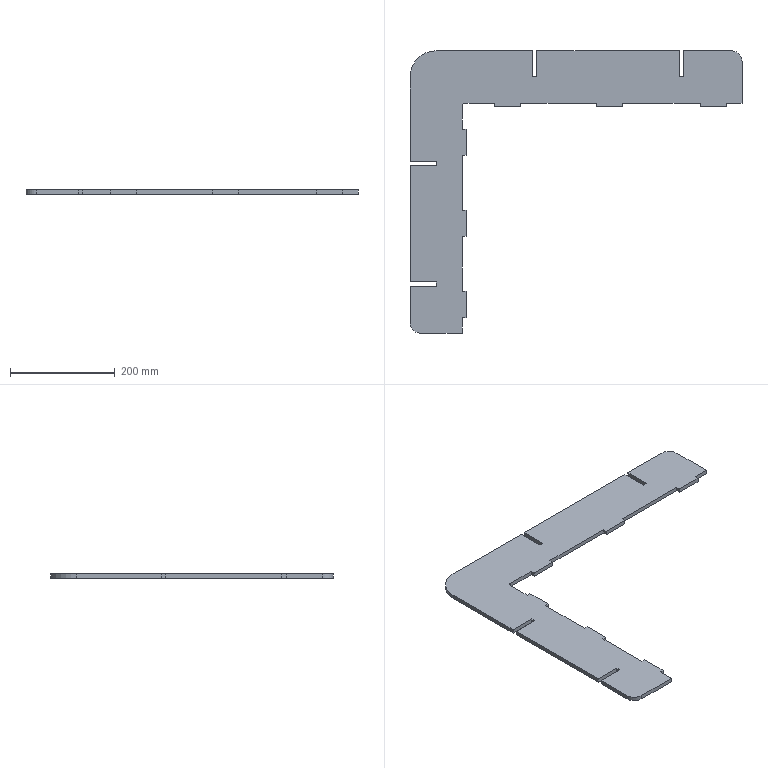Part | SolidWorks | features FlatPattern 1, SMBaseFlange 1, SheetMetal 1 | 1 solid | 52 faces | box 634.6 x 540 x 8 mm | volume 859257 mm3 | plane 48 | cylinder 4 | commonest cylinder face diameters 40 x2 10 x1 100 x1